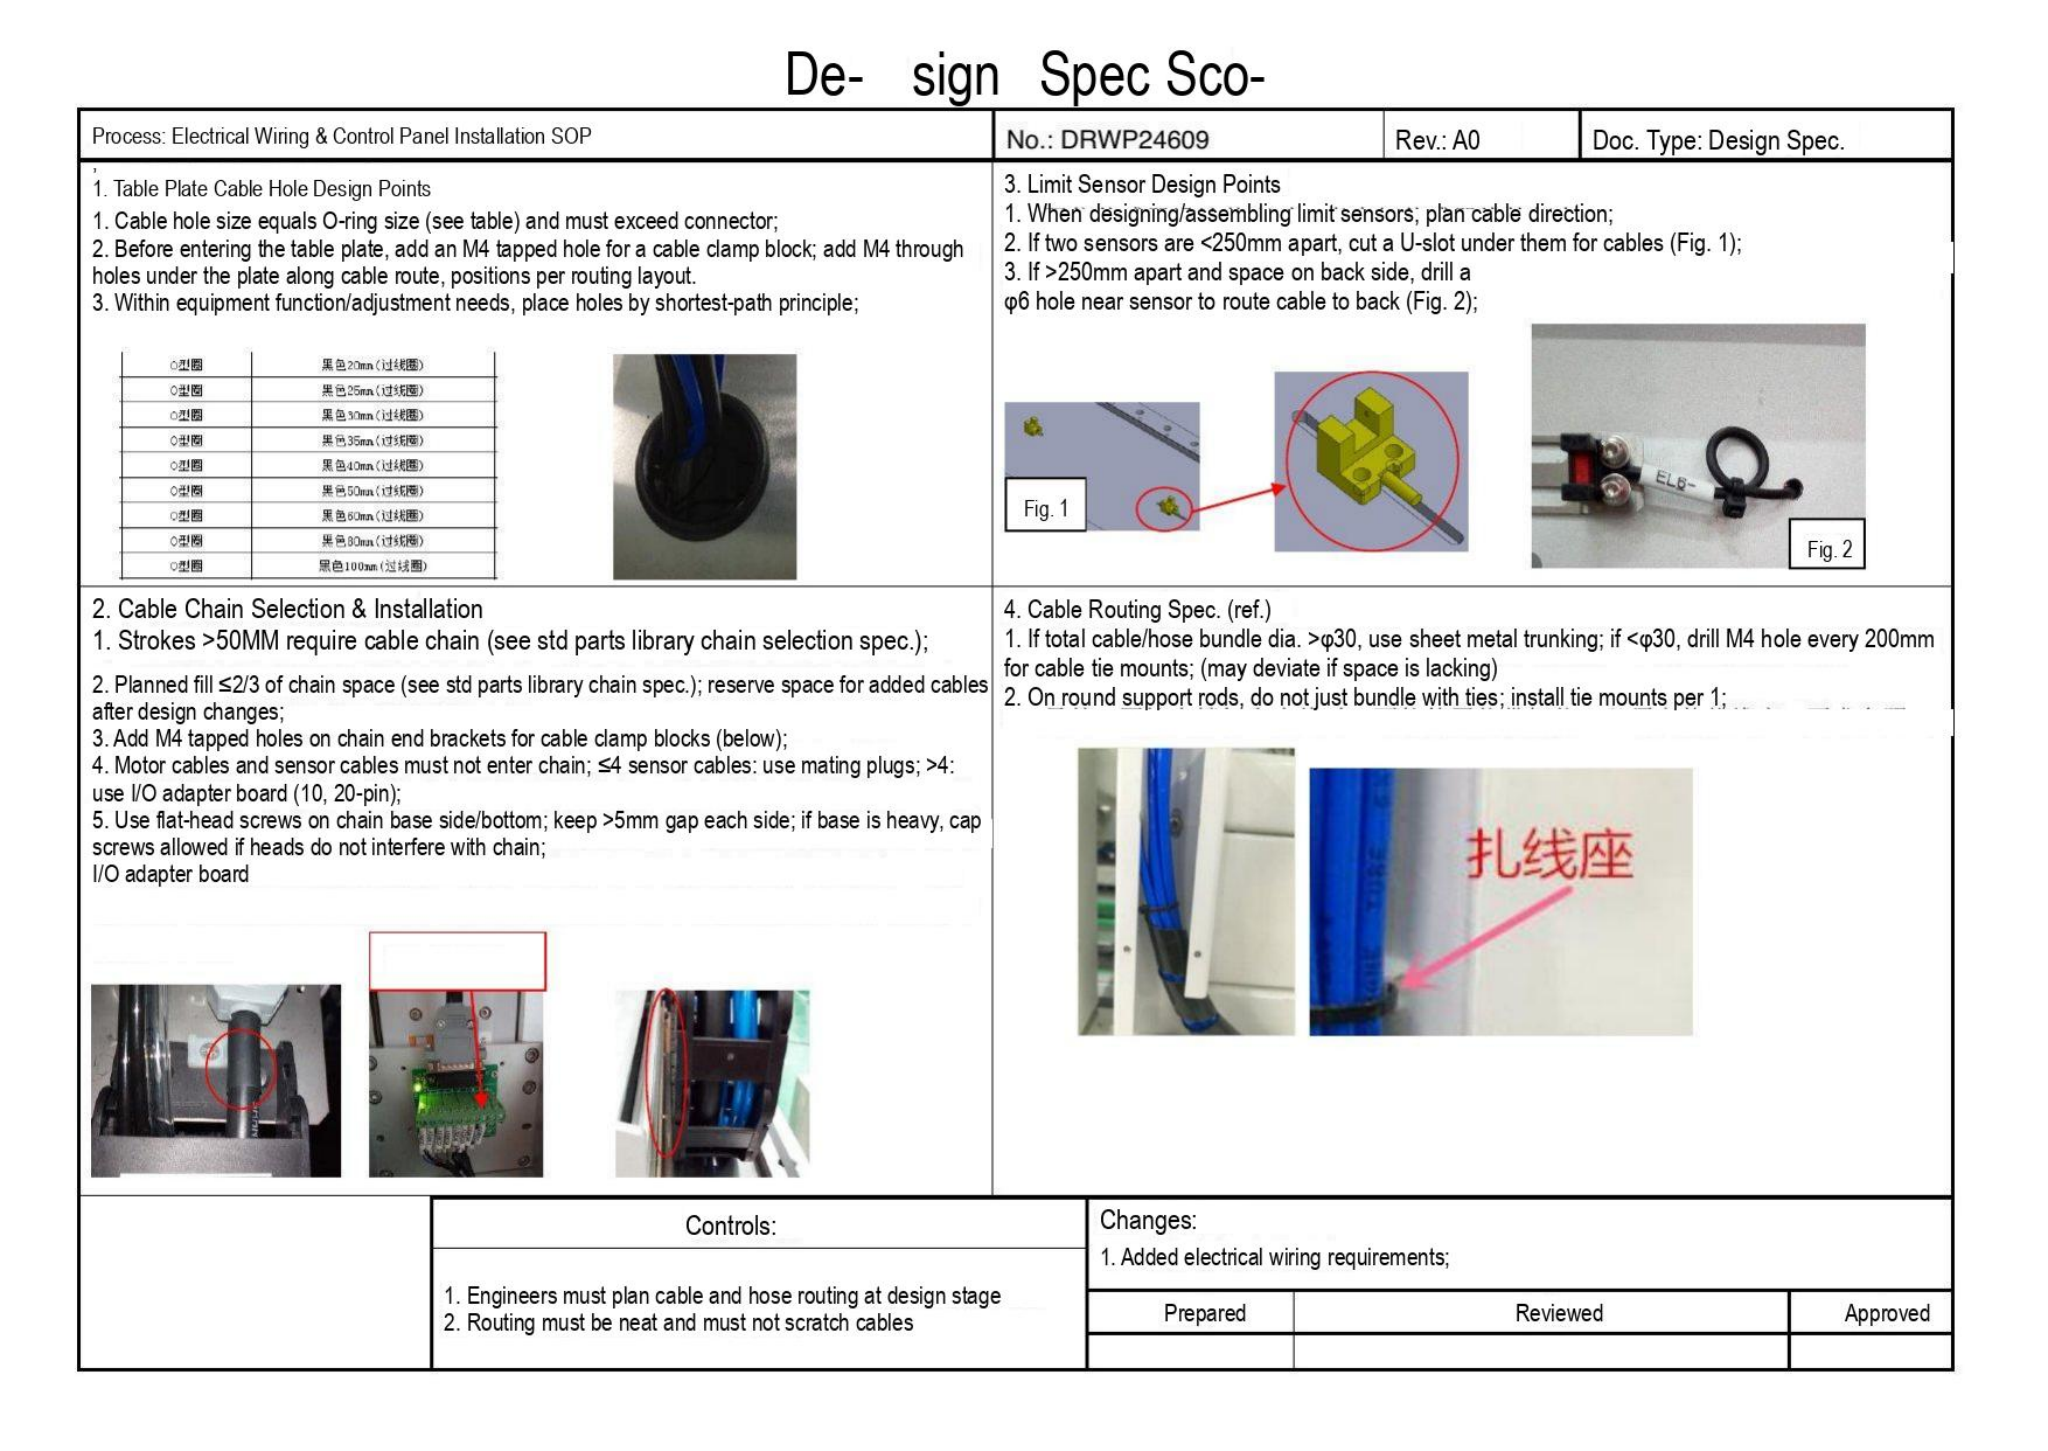# De- sign Spec Sco-

| Process: Electrical Wiring & Control Panel Installation SOP | No.: DRWP24609 | Rev.: A0 | Doc. Type: Design Spec. |
|---|---|---|---|

1. Table Plate Cable Hole Design Points
1. Cable hole size equals O-ring size (see table) and must exceed connector;
2. Before entering the table plate, add an M4 tapped hole for a cable clamp block; add M4 through holes under the plate along cable route, positions per routing layout.
3. Within equipment function/adjustment needs, place holes by shortest-path principle;

| O型圈 | 黑色20mm（过线圈） |
|---|---|
| O型圈 | 黑色25mm（过线圈） |
| O型圈 | 黑色30mm（过线圈） |
| O型圈 | 黑色35mm（过线圈） |
| O型圈 | 黑色40mm（过线圈） |
| O型圈 | 黑色50mm（过线圈） |
| O型圈 | 黑色60mm（过线圈） |
| O型圈 | 黑色80mm（过线圈） |
| O型圈 | 黑色100mm（过线圈） |

3. Limit Sensor Design Points
1. When designing/assembling limit sensors, plan cable direction;
2. If two sensors are <250mm apart, cut a U-slot under them for cables (Fig. 1);
3. If >250mm apart and space on back side, drill a φ6 hole near sensor to route cable to back (Fig. 2);

Fig. 1

ELB-

Fig. 2

2. Cable Chain Selection & Installation
1. Strokes >50MM require cable chain (see std parts library chain selection spec.);
2. Planned fill ≤2/3 of chain space (see std parts library chain spec.); reserve space for added cables after design changes;
3. Add M4 tapped holes on chain end brackets for cable clamp blocks (below);
4. Motor cables and sensor cables must not enter chain; ≤4 sensor cables: use mating plugs; >4: use I/O adapter board (10, 20-pin);
5. Use flat-head screws on chain base side/bottom; keep >5mm gap each side; if base is heavy, cap screws allowed if heads do not interfere with chain;
I/O adapter board

4. Cable Routing Spec. (ref.)
1. If total cable/hose bundle dia. >φ30, use sheet metal trunking; if <φ30, drill M4 hole every 200mm for cable tie mounts; (may deviate if space is lacking)
2. On round support rods, do not just bundle with ties; install tie mounts per 1;

扎线座

Controls:
1. Engineers must plan cable and hose routing at design stage
2. Routing must be neat and must not scratch cables

Changes:
1. Added electrical wiring requirements;

| Prepared | Reviewed | Approved |
|---|---|---|
| | | |
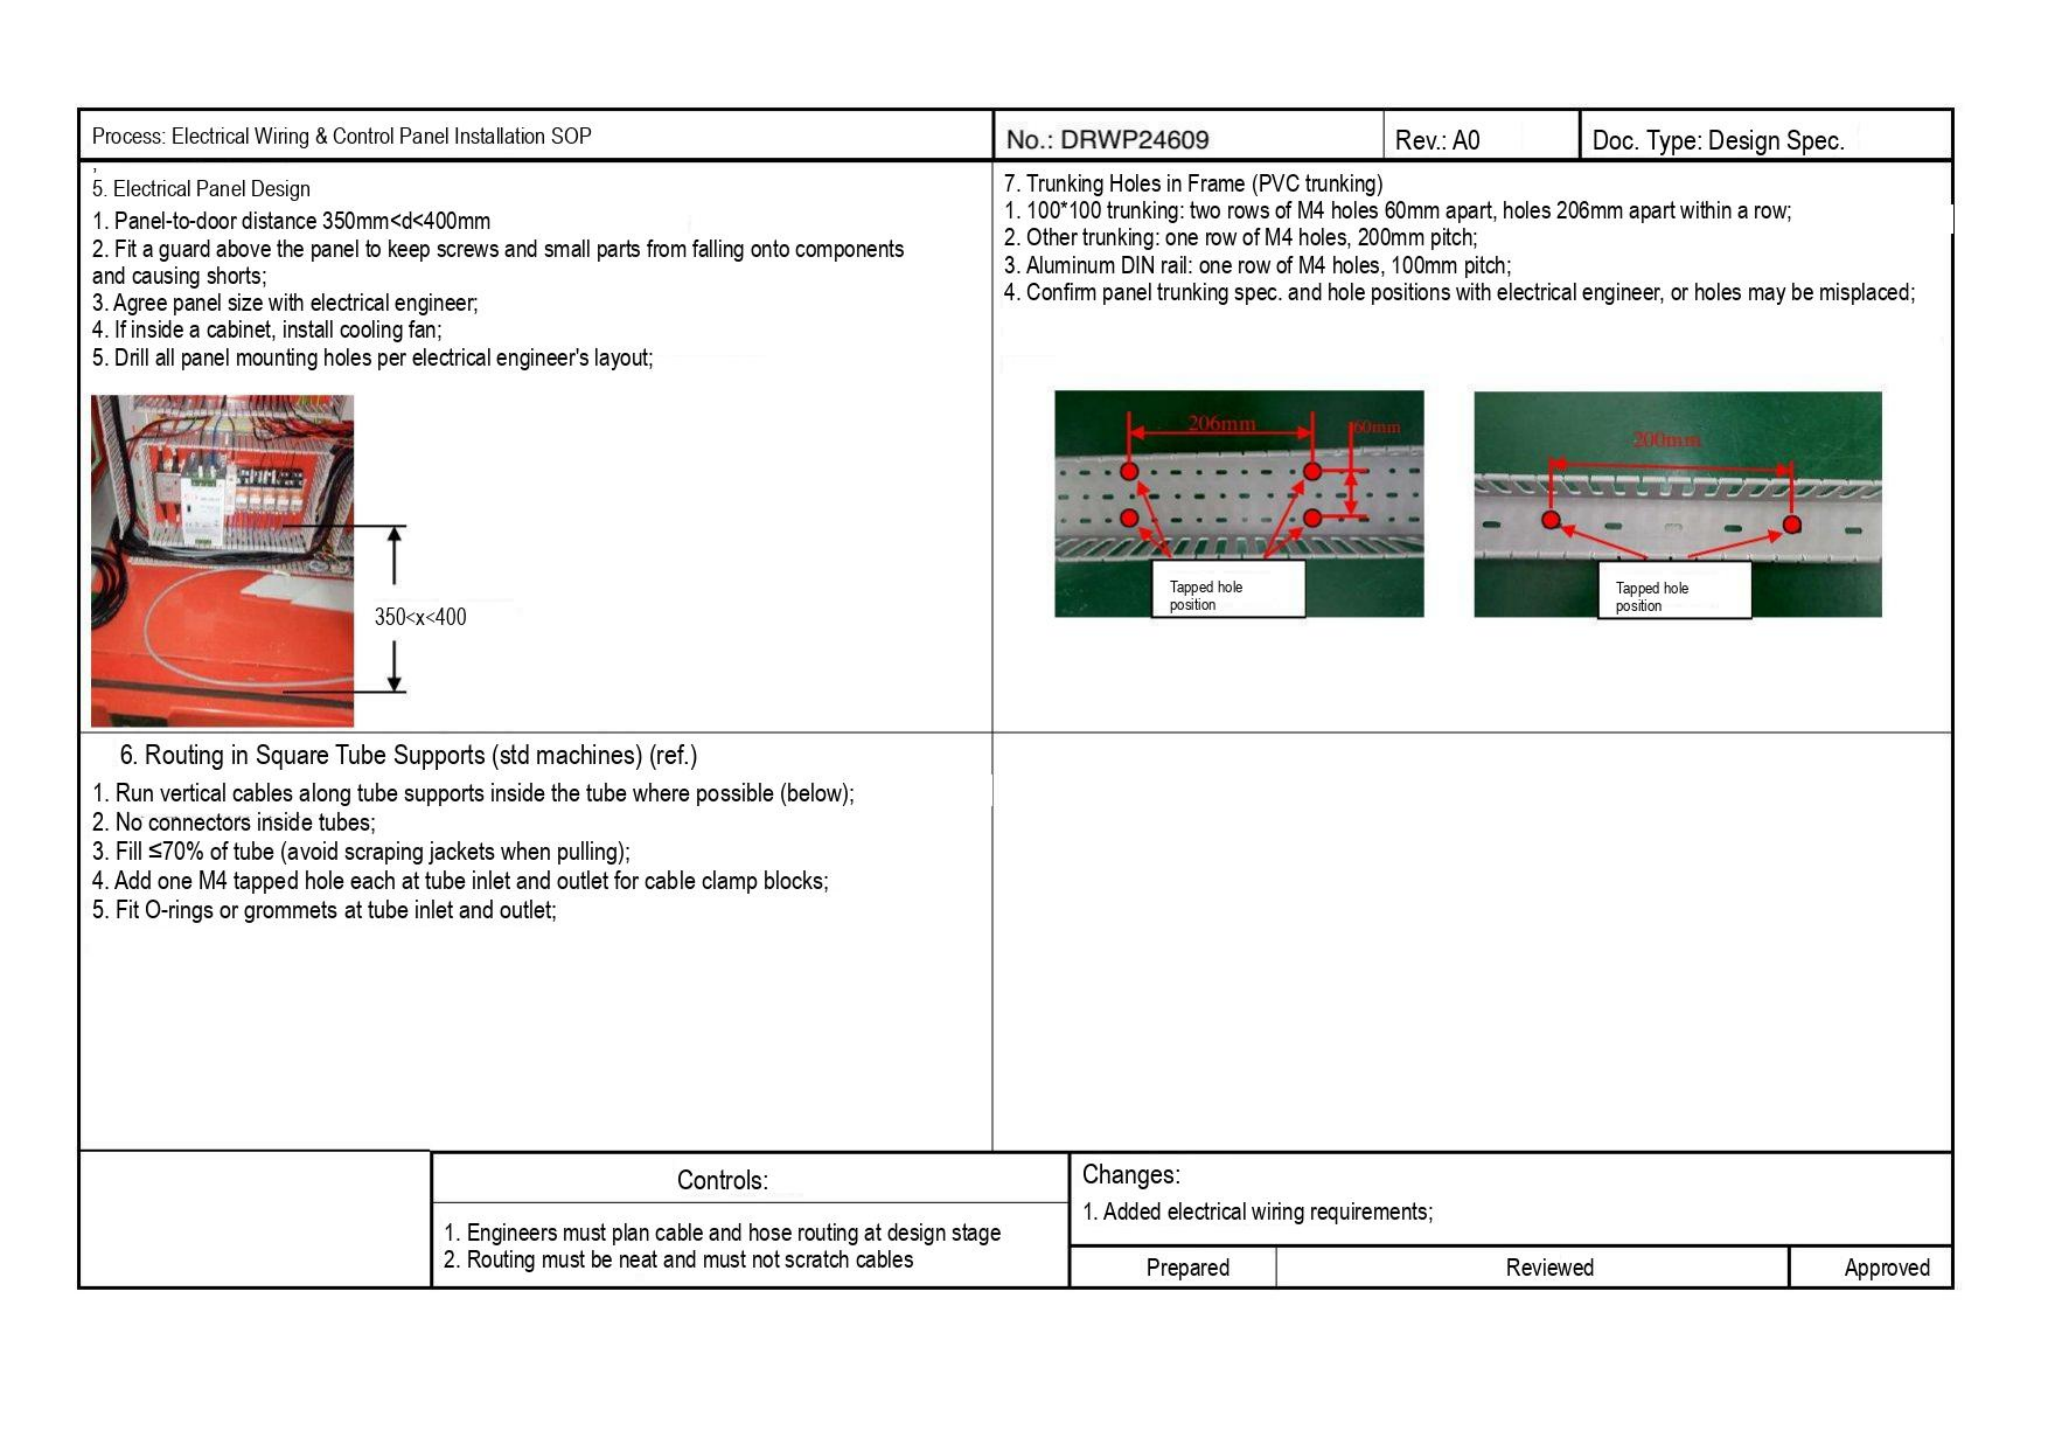Process: Electrical Wiring & Control Panel Installation SOP | No.: DRWP24609 | Rev.: A0 | Doc. Type: Design Spec.

5. Electrical Panel Design
1. Panel-to-door distance 350mm<d<400mm
2. Fit a guard above the panel to keep screws and small parts from falling onto components and causing shorts;
3. Agree panel size with electrical engineer;
4. If inside a cabinet, install cooling fan;
5. Drill all panel mounting holes per electrical engineer's layout;

350<x<400

7. Trunking Holes in Frame (PVC trunking)
1. 100*100 trunking: two rows of M4 holes 60mm apart, holes 206mm apart within a row;
2. Other trunking: one row of M4 holes, 200mm pitch;
3. Aluminum DIN rail: one row of M4 holes, 100mm pitch;
4. Confirm panel trunking spec. and hole positions with electrical engineer, or holes may be misplaced;

206mm
60mm
Tapped hole position

200mm
Tapped hole position

6. Routing in Square Tube Supports (std machines) (ref.)
1. Run vertical cables along tube supports inside the tube where possible (below);
2. No connectors inside tubes;
3. Fill ≤70% of tube (avoid scraping jackets when pulling);
4. Add one M4 tapped hole each at tube inlet and outlet for cable clamp blocks;
5. Fit O-rings or grommets at tube inlet and outlet;

| Controls: | Changes: |
|---|---|
| 1. Engineers must plan cable and hose routing at design stage<br>2. Routing must be neat and must not scratch cables | 1. Added electrical wiring requirements; |

| Prepared | Reviewed | Approved |
|---|---|---|
| | | |